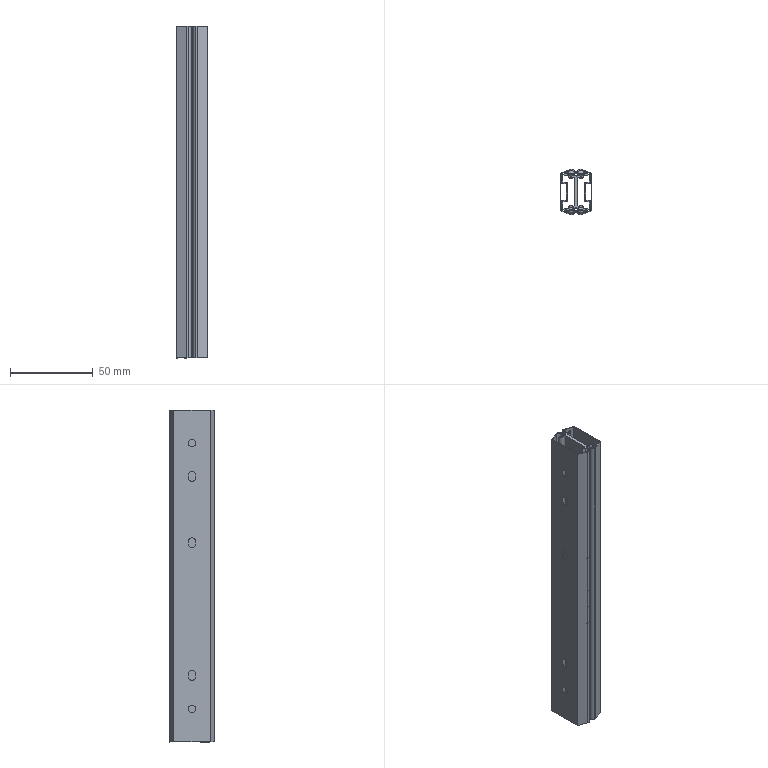Part | SolidWorks | features AEMSimFeature 1 | 5 solids | 208 faces | box 19.1 x 27 x 200 mm | volume 23811 mm3 | plane 88 | spline 70 | cylinder 50 | commonest cylinder face diameters 4.2 x18 3.7 x16 4.5 x8 1 x4 2 x4